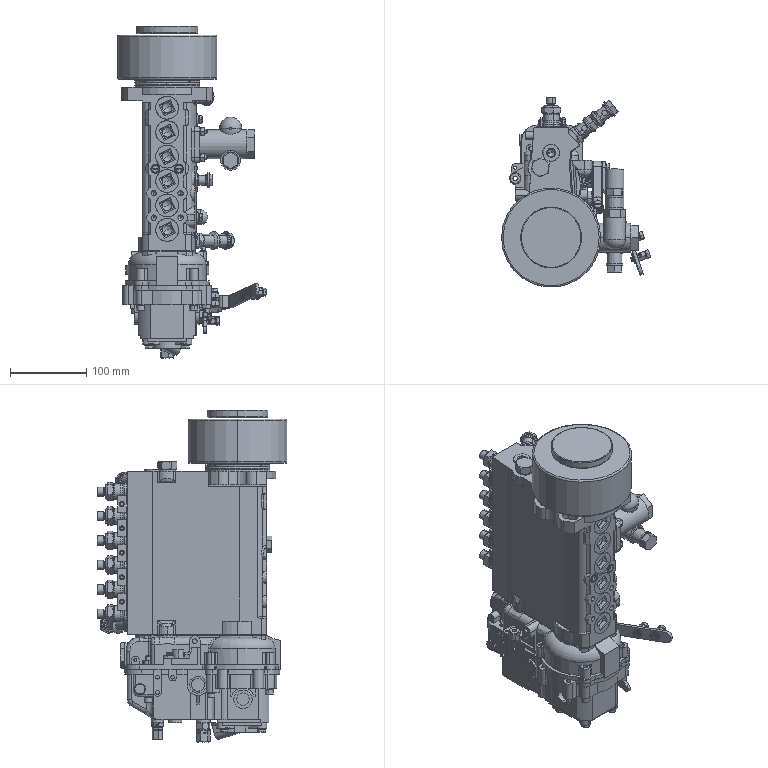Part | SolidWorks | 181 solids | 8045 faces | volume 3189042 mm3 | cylinder 2855 | plane 2701 | cone 2042 | torus 313 | spline 92 | sphere 42 | commonest cylinder face diameters 6 x762 18 x124 10 x118 6.5 x92 20 x87 6.1 x85